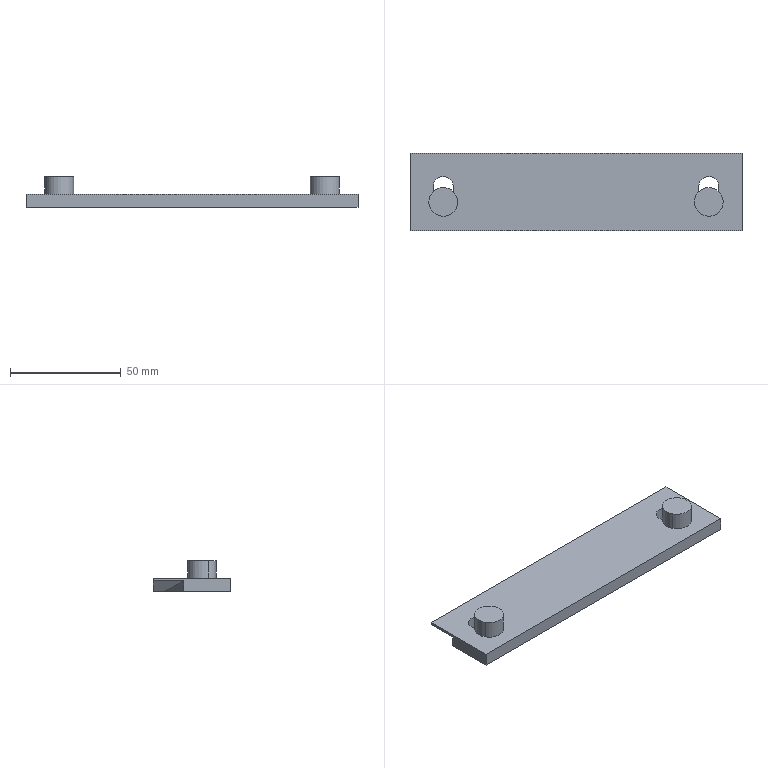Part | CATIA | 3 solids | 26 faces | box 150 x 35 x 14 mm | volume 31317 mm3 | plane 18 | cylinder 8 | commonest cylinder face diameters 9 x4 13 x4
STEP:
#1=CARTESIAN_POINT('',(-75.,-30.,38.));
#2=VERTEX_POINT('',#1);
#3=CARTESIAN_POINT('',(-75.,-30.,44.));
#4=VERTEX_POINT('',#3);
#5=CARTESIAN_POINT('',(-75.,-30.,41.));
#6=DIRECTION('',(0.,0.,1.));
#7=VECTOR('',#6,1.);
#8=LINE('',#5,#7);
#9=EDGE_CURVE('',#2,#4,#8,.T.);
#10=ORIENTED_EDGE('',*,*,#9,.F.);
#11=CARTESIAN_POINT('',(75.,-30.,38.));
#12=VERTEX_POINT('',#11);
#13=CARTESIAN_POINT('',(0.,-30.,38.));
#14=DIRECTION('',(1.,0.,0.));
#15=VECTOR('',#14,1.);
#16=LINE('',#13,#15);
#17=EDGE_CURVE('',#2,#12,#16,.T.);
#18=ORIENTED_EDGE('',*,*,#17,.T.);
#19=CARTESIAN_POINT('',(75.,-30.,44.));
#20=VERTEX_POINT('',#19);
#21=CARTESIAN_POINT('',(75.,-30.,41.));
#22=DIRECTION('',(0.,0.,1.));
#23=VECTOR('',#22,1.);
#24=LINE('',#21,#23);
#25=EDGE_CURVE('',#12,#20,#24,.T.);
#26=ORIENTED_EDGE('',*,*,#25,.T.);
#27=CARTESIAN_POINT('',(0.,-30.,44.));
#28=DIRECTION('',(1.,0.,0.));
#29=VECTOR('',#28,1.);
#30=LINE('',#27,#29);
#31=EDGE_CURVE('',#4,#20,#30,.T.);
#32=ORIENTED_EDGE('',*,*,#31,.F.);
#33=EDGE_LOOP('',(#10,#18,#26,#32));
#34=FACE_OUTER_BOUND('',#33,.T.);
#35=CARTESIAN_POINT('',(-75.,-30.,38.));
#36=DIRECTION('',(0.,-1.,0.));
#37=DIRECTION('',(1.,0.,0.));
#38=AXIS2_PLACEMENT_3D('',#35,#36,#37);
#39=PLANE('',#38);
#40=ADVANCED_FACE('',(#34),#39,.T.);
#41=CARTESIAN_POINT('',(75.,-8.66,42.874));
#42=VERTEX_POINT('',#41);
#43=CARTESIAN_POINT('',(75.,-8.66,38.));
#44=VERTEX_POINT('',#43);
#45=CARTESIAN_POINT('',(75.,-8.66,40.437));
#46=DIRECTION('',(0.,0.,-1.));
#47=VECTOR('',#46,1.);
#48=LINE('',#45,#47);
#49=EDGE_CURVE('',#42,#44,#48,.T.);
#50=ORIENTED_EDGE('',*,*,#49,.F.);
#51=CARTESIAN_POINT('',(75.,5.,42.874));
#52=VERTEX_POINT('',#51);
#53=CARTESIAN_POINT('',(75.,-1.83,42.874));
#54=DIRECTION('',(0.,1.,0.));
#55=VECTOR('',#54,1.);
#56=LINE('',#53,#55);
#57=EDGE_CURVE('',#42,#52,#56,.T.);
#58=ORIENTED_EDGE('',*,*,#57,.T.);
#59=CARTESIAN_POINT('',(75.,5.,44.));
#60=VERTEX_POINT('',#59);
#61=CARTESIAN_POINT('',(75.,5.,43.437));
#62=DIRECTION('',(0.,0.,1.));
#63=VECTOR('',#62,1.);
#64=LINE('',#61,#63);
#65=EDGE_CURVE('',#52,#60,#64,.T.);
#66=ORIENTED_EDGE('',*,*,#65,.T.);
#67=CARTESIAN_POINT('',(75.,-12.5,44.));
#68=DIRECTION('',(0.,-1.,0.));
#69=VECTOR('',#68,1.);
#70=LINE('',#67,#69);
#71=EDGE_CURVE('',#20,#60,#70,.F.);
#72=ORIENTED_EDGE('',*,*,#71,.F.);
#73=ORIENTED_EDGE('',*,*,#25,.F.);
#74=CARTESIAN_POINT('',(75.,-19.33,38.));
#75=DIRECTION('',(0.,-1.,0.));
#76=VECTOR('',#75,1.);
#77=LINE('',#74,#76);
#78=EDGE_CURVE('',#12,#44,#77,.F.);
#79=ORIENTED_EDGE('',*,*,#78,.T.);
#80=EDGE_LOOP('',(#50,#58,#66,#72,#73,#79));
#81=FACE_OUTER_BOUND('',#80,.T.);
#82=CARTESIAN_POINT('',(75.,5.,38.));
#83=DIRECTION('',(-1.,0.,0.));
#84=DIRECTION('',(0.,-1.,0.));
#85=AXIS2_PLACEMENT_3D('',#82,#83,#84);
#86=PLANE('',#85);
#87=ADVANCED_FACE('',(#81),#86,.F.);
#88=CARTESIAN_POINT('',(-75.,-8.66,42.874));
#89=VERTEX_POINT('',#88);
#90=CARTESIAN_POINT('',(-75.,5.,42.874));
#91=VERTEX_POINT('',#90);
#92=CARTESIAN_POINT('',(-75.,-1.83,42.874));
#93=DIRECTION('',(0.,1.,0.));
#94=VECTOR('',#93,1.);
#95=LINE('',#92,#94);
#96=EDGE_CURVE('',#89,#91,#95,.T.);
#97=ORIENTED_EDGE('',*,*,#96,.F.);
#98=CARTESIAN_POINT('',(-75.,-8.66,38.));
#99=VERTEX_POINT('',#98);
#100=CARTESIAN_POINT('',(-75.,-8.66,40.437));
#101=DIRECTION('',(0.,0.,-1.));
#102=VECTOR('',#101,1.);
#103=LINE('',#100,#102);
#104=EDGE_CURVE('',#89,#99,#103,.T.);
#105=ORIENTED_EDGE('',*,*,#104,.T.);
#106=CARTESIAN_POINT('',(-75.,-19.33,38.));
#107=DIRECTION('',(0.,1.,0.));
#108=VECTOR('',#107,1.);
#109=LINE('',#106,#108);
#110=EDGE_CURVE('',#99,#2,#109,.F.);
#111=ORIENTED_EDGE('',*,*,#110,.T.);
#112=ORIENTED_EDGE('',*,*,#9,.T.);
#113=CARTESIAN_POINT('',(-75.,5.,44.));
#114=VERTEX_POINT('',#113);
#115=CARTESIAN_POINT('',(-75.,-12.5,44.));
#116=DIRECTION('',(0.,1.,0.));
#117=VECTOR('',#116,1.);
#118=LINE('',#115,#117);
#119=EDGE_CURVE('',#114,#4,#118,.F.);
#120=ORIENTED_EDGE('',*,*,#119,.F.);
#121=CARTESIAN_POINT('',(-75.,5.,43.437));
#122=DIRECTION('',(0.,0.,1.));
#123=VECTOR('',#122,1.);
#124=LINE('',#121,#123);
#125=EDGE_CURVE('',#91,#114,#124,.T.);
#126=ORIENTED_EDGE('',*,*,#125,.F.);
#127=EDGE_LOOP('',(#97,#105,#111,#112,#120,#126));
#128=FACE_OUTER_BOUND('',#127,.T.);
#129=CARTESIAN_POINT('',(-75.,-30.,38.));
#130=DIRECTION('',(1.,0.,0.));
#131=DIRECTION('',(0.,1.,0.));
#132=AXIS2_PLACEMENT_3D('',#129,#130,#131);
#133=PLANE('',#132);
#134=ADVANCED_FACE('',(#128),#133,.F.);
#135=CARTESIAN_POINT('',(60.,5.,38.));
#136=VERTEX_POINT('',#135);
#137=CARTESIAN_POINT('',(-60.,5.,38.));
#138=VERTEX_POINT('',#137);
#139=CARTESIAN_POINT('',(0.,5.,38.));
#140=DIRECTION('',(-1.,0.,0.));
#141=VECTOR('',#140,1.);
#142=LINE('',#139,#141);
#143=EDGE_CURVE('',#136,#138,#142,.T.);
#144=ORIENTED_EDGE('',*,*,#143,.T.);
#145=CARTESIAN_POINT('',(-67.5,5.,40.437));
#146=DIRECTION('',(-0.9511,0.,0.309));
#147=VECTOR('',#146,1.);
#148=LINE('',#145,#147);
#149=EDGE_CURVE('',#138,#91,#148,.T.);
#150=ORIENTED_EDGE('',*,*,#149,.T.);
#151=ORIENTED_EDGE('',*,*,#125,.T.);
#152=CARTESIAN_POINT('',(0.,5.,44.));
#153=DIRECTION('',(-1.,0.,0.));
#154=VECTOR('',#153,1.);
#155=LINE('',#152,#154);
#156=EDGE_CURVE('',#60,#114,#155,.T.);
#157=ORIENTED_EDGE('',*,*,#156,.F.);
#158=ORIENTED_EDGE('',*,*,#65,.F.);
#159=CARTESIAN_POINT('',(67.5,5.,40.437));
#160=DIRECTION('',(0.9511,0.,0.309));
#161=VECTOR('',#160,1.);
#162=LINE('',#159,#161);
#163=EDGE_CURVE('',#136,#52,#162,.T.);
#164=ORIENTED_EDGE('',*,*,#163,.F.);
#165=EDGE_LOOP('',(#144,#150,#151,#157,#158,#164));
#166=FACE_OUTER_BOUND('',#165,.T.);
#167=CARTESIAN_POINT('',(75.,5.,38.));
#168=DIRECTION('',(0.,1.,0.));
#169=DIRECTION('',(-1.,0.,0.));
#170=AXIS2_PLACEMENT_3D('',#167,#168,#169);
#171=PLANE('',#170);
#172=ADVANCED_FACE('',(#166),#171,.T.);
#173=CARTESIAN_POINT('',(60.,0.,38.));
#174=VERTEX_POINT('',#173);
#175=CARTESIAN_POINT('',(75.,-8.66,42.874));
#176=CARTESIAN_POINT('',(60.,0.,38.));
#177=B_SPLINE_CURVE_WITH_KNOTS('',1,(#175,#176),.UNSPECIFIED.,.F.,.U.,(2,2),(-2.999,14.994),.UNSPECIFIED.);
#178=EDGE_CURVE('',#174,#42,#177,.F.);
#179=ORIENTED_EDGE('',*,*,#178,.T.);
#180=ORIENTED_EDGE('',*,*,#49,.T.);
#181=CARTESIAN_POINT('',(72.5,-7.217,38.));
#182=DIRECTION('',(0.866,-0.5,0.));
#183=VECTOR('',#182,1.);
#184=LINE('',#181,#183);
#185=EDGE_CURVE('',#174,#44,#184,.T.);
#186=ORIENTED_EDGE('',*,*,#185,.F.);
#187=EDGE_LOOP('',(#179,#180,#186));
#188=FACE_OUTER_BOUND('',#187,.T.);
#189=CARTESIAN_POINT('',(60.,0.,38.));
#190=DIRECTION('',(0.5,0.866,0.));
#191=DIRECTION('',(0.,0.,1.));
#192=AXIS2_PLACEMENT_3D('',#189,#190,#191);
#193=PLANE('',#192);
#194=ADVANCED_FACE('',(#188),#193,.T.);
#195=ORIENTED_EDGE('',*,*,#163,.T.);
#196=ORIENTED_EDGE('',*,*,#57,.F.);
#197=ORIENTED_EDGE('',*,*,#178,.F.);
#198=CARTESIAN_POINT('',(60.,5.,38.));
#199=DIRECTION('',(0.,-1.,0.));
#200=VECTOR('',#199,1.);
#201=LINE('',#198,#200);
#202=EDGE_CURVE('',#174,#136,#201,.F.);
#203=ORIENTED_EDGE('',*,*,#202,.T.);
#204=EDGE_LOOP('',(#195,#196,#197,#203));
#205=FACE_OUTER_BOUND('',#204,.T.);
#206=CARTESIAN_POINT('',(60.,10.,38.));
#207=DIRECTION('',(-0.309,0.,0.9511));
#208=DIRECTION('',(0.,-1.,0.));
#209=AXIS2_PLACEMENT_3D('',#206,#207,#208);
#210=PLANE('',#209);
#211=ADVANCED_FACE('',(#205),#210,.F.);
#212=CARTESIAN_POINT('',(-60.,0.,38.));
#213=VERTEX_POINT('',#212);
#214=CARTESIAN_POINT('',(-72.5,-7.217,38.));
#215=DIRECTION('',(-0.866,-0.5,0.));
#216=VECTOR('',#215,1.);
#217=LINE('',#214,#216);
#218=EDGE_CURVE('',#213,#99,#217,.T.);
#219=ORIENTED_EDGE('',*,*,#218,.T.);
#220=ORIENTED_EDGE('',*,*,#104,.F.);
#221=CARTESIAN_POINT('',(-75.,-8.66,42.874));
#222=CARTESIAN_POINT('',(-60.,0.,38.));
#223=B_SPLINE_CURVE_WITH_KNOTS('',1,(#221,#222),.UNSPECIFIED.,.F.,.U.,(2,2),(-2.999,14.994),.UNSPECIFIED.);
#224=EDGE_CURVE('',#213,#89,#223,.F.);
#225=ORIENTED_EDGE('',*,*,#224,.F.);
#226=EDGE_LOOP('',(#219,#220,#225));
#227=FACE_OUTER_BOUND('',#226,.T.);
#228=CARTESIAN_POINT('',(-60.,0.,38.));
#229=DIRECTION('',(0.5,-0.866,0.));
#230=DIRECTION('',(0.,0.,1.));
#231=AXIS2_PLACEMENT_3D('',#228,#229,#230);
#232=PLANE('',#231);
#233=ADVANCED_FACE('',(#227),#232,.F.);
#234=CARTESIAN_POINT('',(-60.,5.,38.));
#235=DIRECTION('',(0.,-1.,0.));
#236=VECTOR('',#235,1.);
#237=LINE('',#234,#236);
#238=EDGE_CURVE('',#213,#138,#237,.F.);
#239=ORIENTED_EDGE('',*,*,#238,.F.);
#240=ORIENTED_EDGE('',*,*,#224,.T.);
#241=ORIENTED_EDGE('',*,*,#96,.T.);
#242=ORIENTED_EDGE('',*,*,#149,.F.);
#243=EDGE_LOOP('',(#239,#240,#241,#242));
#244=FACE_OUTER_BOUND('',#243,.T.);
#245=CARTESIAN_POINT('',(-60.,10.,38.));
#246=DIRECTION('',(-0.309,0.,-0.9511));
#247=DIRECTION('',(0.,-1.,0.));
#248=AXIS2_PLACEMENT_3D('',#245,#246,#247);
#249=PLANE('',#248);
#250=ADVANCED_FACE('',(#244),#249,.T.);
#251=ORIENTED_EDGE('',*,*,#143,.F.);
#252=ORIENTED_EDGE('',*,*,#202,.F.);
#253=ORIENTED_EDGE('',*,*,#185,.T.);
#254=ORIENTED_EDGE('',*,*,#78,.F.);
#255=ORIENTED_EDGE('',*,*,#17,.F.);
#256=ORIENTED_EDGE('',*,*,#110,.F.);
#257=ORIENTED_EDGE('',*,*,#218,.F.);
#258=ORIENTED_EDGE('',*,*,#238,.T.);
#259=EDGE_LOOP('',(#251,#252,#253,#254,#255,#256,#257,#258));
#260=FACE_OUTER_BOUND('',#259,.T.);
#261=CARTESIAN_POINT('',(-55.5,-10.,38.));
#262=VERTEX_POINT('',#261);
#263=CARTESIAN_POINT('',(-55.5,-17.,38.));
#264=VERTEX_POINT('',#263);
#265=CARTESIAN_POINT('',(-55.5,-13.5,38.));
#266=DIRECTION('',(0.,-1.,0.));
#267=VECTOR('',#266,1.);
#268=LINE('',#265,#267);
#269=EDGE_CURVE('',#262,#264,#268,.T.);
#270=ORIENTED_EDGE('',*,*,#269,.F.);
#271=CARTESIAN_POINT('',(-64.5,-10.,38.));
#272=VERTEX_POINT('',#271);
#273=CARTESIAN_POINT('',(-60.,-10.,38.));
#274=DIRECTION('',(0.,0.,1.));
#275=AXIS2_PLACEMENT_3D('',#273,#274,$);
#276=CIRCLE('',#275,4.5);
#277=EDGE_CURVE('',#262,#272,#276,.T.);
#278=ORIENTED_EDGE('',*,*,#277,.T.);
#279=CARTESIAN_POINT('',(-64.5,-17.,38.));
#280=VERTEX_POINT('',#279);
#281=CARTESIAN_POINT('',(-64.5,-13.5,38.));
#282=DIRECTION('',(0.,-1.,0.));
#283=VECTOR('',#282,1.);
#284=LINE('',#281,#283);
#285=EDGE_CURVE('',#272,#280,#284,.T.);
#286=ORIENTED_EDGE('',*,*,#285,.T.);
#287=CARTESIAN_POINT('',(-60.,-17.,38.));
#288=DIRECTION('',(0.,0.,1.));
#289=AXIS2_PLACEMENT_3D('',#287,#288,$);
#290=CIRCLE('',#289,4.5);
#291=EDGE_CURVE('',#280,#264,#290,.T.);
#292=ORIENTED_EDGE('',*,*,#291,.T.);
#293=EDGE_LOOP('',(#270,#278,#286,#292));
#294=FACE_BOUND('',#293,.T.);
#295=CARTESIAN_POINT('',(64.5,-10.,38.));
#296=VERTEX_POINT('',#295);
#297=CARTESIAN_POINT('',(55.5,-10.,38.));
#298=VERTEX_POINT('',#297);
#299=CARTESIAN_POINT('',(60.,-10.,38.));
#300=DIRECTION('',(0.,0.,1.));
#301=AXIS2_PLACEMENT_3D('',#299,#300,$);
#302=CIRCLE('',#301,4.5);
#303=EDGE_CURVE('',#296,#298,#302,.T.);
#304=ORIENTED_EDGE('',*,*,#303,.T.);
#305=CARTESIAN_POINT('',(55.5,-17.,38.));
#306=VERTEX_POINT('',#305);
#307=CARTESIAN_POINT('',(55.5,-13.5,38.));
#308=DIRECTION('',(0.,-1.,0.));
#309=VECTOR('',#308,1.);
#310=LINE('',#307,#309);
#311=EDGE_CURVE('',#298,#306,#310,.T.);
#312=ORIENTED_EDGE('',*,*,#311,.T.);
#313=CARTESIAN_POINT('',(64.5,-17.,38.));
#314=VERTEX_POINT('',#313);
#315=CARTESIAN_POINT('',(60.,-17.,38.));
#316=DIRECTION('',(0.,0.,1.));
#317=AXIS2_PLACEMENT_3D('',#315,#316,$);
#318=CIRCLE('',#317,4.5);
#319=EDGE_CURVE('',#306,#314,#318,.T.);
#320=ORIENTED_EDGE('',*,*,#319,.T.);
#321=CARTESIAN_POINT('',(64.5,-13.5,38.));
#322=DIRECTION('',(0.,-1.,0.));
#323=VECTOR('',#322,1.);
#324=LINE('',#321,#323);
#325=EDGE_CURVE('',#296,#314,#324,.T.);
#326=ORIENTED_EDGE('',*,*,#325,.F.);
#327=EDGE_LOOP('',(#304,#312,#320,#326));
#328=FACE_BOUND('',#327,.T.);
#329=CARTESIAN_POINT('',(0.,0.,38.));
#330=DIRECTION('',(0.,0.,1.));
#331=DIRECTION('',(1.,0.,0.));
#332=AXIS2_PLACEMENT_3D('',#329,#330,#331);
#333=PLANE('',#332);
#334=ADVANCED_FACE('',(#260,#294,#328),#333,.F.);
#335=ORIENTED_EDGE('',*,*,#156,.T.);
#336=ORIENTED_EDGE('',*,*,#119,.T.);
#337=ORIENTED_EDGE('',*,*,#31,.T.);
#338=ORIENTED_EDGE('',*,*,#71,.T.);
#339=EDGE_LOOP('',(#335,#336,#337,#338));
#340=FACE_OUTER_BOUND('',#339,.T.);
#341=CARTESIAN_POINT('',(-55.5,-17.,44.));
#342=VERTEX_POINT('',#341);
#343=CARTESIAN_POINT('',(-55.5,-10.,44.));
#344=VERTEX_POINT('',#343);
#345=CARTESIAN_POINT('',(-55.5,-13.5,44.));
#346=DIRECTION('',(0.,-1.,0.));
#347=VECTOR('',#346,1.);
#348=LINE('',#345,#347);
#349=EDGE_CURVE('',#342,#344,#348,.F.);
#350=ORIENTED_EDGE('',*,*,#349,.F.);
#351=CARTESIAN_POINT('',(-64.5,-17.,44.));
#352=VERTEX_POINT('',#351);
#353=CARTESIAN_POINT('',(-60.,-17.,44.));
#354=DIRECTION('',(0.,0.,1.));
#355=AXIS2_PLACEMENT_3D('',#353,#354,$);
#356=CIRCLE('',#355,4.5);
#357=EDGE_CURVE('',#352,#342,#356,.T.);
#358=ORIENTED_EDGE('',*,*,#357,.F.);
#359=CARTESIAN_POINT('',(-64.5,-10.,44.));
#360=VERTEX_POINT('',#359);
#361=CARTESIAN_POINT('',(-64.5,-13.5,44.));
#362=DIRECTION('',(0.,-1.,0.));
#363=VECTOR('',#362,1.);
#364=LINE('',#361,#363);
#365=EDGE_CURVE('',#360,#352,#364,.T.);
#366=ORIENTED_EDGE('',*,*,#365,.F.);
#367=CARTESIAN_POINT('',(-60.,-10.,44.));
#368=DIRECTION('',(0.,0.,1.));
#369=AXIS2_PLACEMENT_3D('',#367,#368,$);
#370=CIRCLE('',#369,4.5);
#371=EDGE_CURVE('',#344,#360,#370,.T.);
#372=ORIENTED_EDGE('',*,*,#371,.F.);
#373=EDGE_LOOP('',(#350,#358,#366,#372));
#374=FACE_BOUND('',#373,.T.);
#375=CARTESIAN_POINT('',(64.5,-10.,44.));
#376=VERTEX_POINT('',#375);
#377=CARTESIAN_POINT('',(55.5,-10.,44.));
#378=VERTEX_POINT('',#377);
#379=CARTESIAN_POINT('',(60.,-10.,44.));
#380=DIRECTION('',(0.,0.,1.));
#381=AXIS2_PLACEMENT_3D('',#379,#380,$);
#382=CIRCLE('',#381,4.5);
#383=EDGE_CURVE('',#376,#378,#382,.T.);
#384=ORIENTED_EDGE('',*,*,#383,.F.);
#385=CARTESIAN_POINT('',(64.5,-17.,44.));
#386=VERTEX_POINT('',#385);
#387=CARTESIAN_POINT('',(64.5,-13.5,44.));
#388=DIRECTION('',(0.,-1.,0.));
#389=VECTOR('',#388,1.);
#390=LINE('',#387,#389);
#391=EDGE_CURVE('',#386,#376,#390,.F.);
#392=ORIENTED_EDGE('',*,*,#391,.F.);
#393=CARTESIAN_POINT('',(55.5,-17.,44.));
#394=VERTEX_POINT('',#393);
#395=CARTESIAN_POINT('',(60.,-17.,44.));
#396=DIRECTION('',(0.,0.,1.));
#397=AXIS2_PLACEMENT_3D('',#395,#396,$);
#398=CIRCLE('',#397,4.5);
#399=EDGE_CURVE('',#394,#386,#398,.T.);
#400=ORIENTED_EDGE('',*,*,#399,.F.);
#401=CARTESIAN_POINT('',(55.5,-13.5,44.));
#402=DIRECTION('',(0.,-1.,0.));
#403=VECTOR('',#402,1.);
#404=LINE('',#401,#403);
#405=EDGE_CURVE('',#378,#394,#404,.T.);
#406=ORIENTED_EDGE('',*,*,#405,.F.);
#407=EDGE_LOOP('',(#384,#392,#400,#406));
#408=FACE_BOUND('',#407,.T.);
#409=CARTESIAN_POINT('',(0.,0.,44.));
#410=DIRECTION('',(0.,0.,1.));
#411=DIRECTION('',(1.,0.,0.));
#412=AXIS2_PLACEMENT_3D('',#409,#410,#411);
#413=PLANE('',#412);
#414=ADVANCED_FACE('',(#340,#374,#408),#413,.T.);
#415=ORIENTED_EDGE('',*,*,#303,.F.);
#416=CARTESIAN_POINT('',(64.5,-10.,34.));
#417=DIRECTION('',(0.,0.,1.));
#418=VECTOR('',#417,1.);
#419=LINE('',#416,#418);
#420=EDGE_CURVE('',#376,#296,#419,.F.);
#421=ORIENTED_EDGE('',*,*,#420,.F.);
#422=ORIENTED_EDGE('',*,*,#383,.T.);
#423=CARTESIAN_POINT('',(55.5,-10.,34.));
#424=DIRECTION('',(0.,0.,1.));
#425=VECTOR('',#424,1.);
#426=LINE('',#423,#425);
#427=EDGE_CURVE('',#378,#298,#426,.F.);
#428=ORIENTED_EDGE('',*,*,#427,.T.);
#429=EDGE_LOOP('',(#415,#421,#422,#428));
#430=FACE_OUTER_BOUND('',#429,.T.);
#431=CARTESIAN_POINT('',(60.,-10.,34.));
#432=DIRECTION('',(0.,0.,1.));
#433=DIRECTION('',(1.,0.,0.));
#434=AXIS2_PLACEMENT_3D('',#431,#432,#433);
#435=CYLINDRICAL_SURFACE('',#434,4.5);
#436=ADVANCED_FACE('',(#430),#435,.F.);
#437=ORIENTED_EDGE('',*,*,#427,.F.);
#438=ORIENTED_EDGE('',*,*,#405,.T.);
#439=CARTESIAN_POINT('',(55.5,-17.,41.));
#440=DIRECTION('',(0.,0.,-1.));
#441=VECTOR('',#440,1.);
#442=LINE('',#439,#441);
#443=EDGE_CURVE('',#394,#306,#442,.T.);
#444=ORIENTED_EDGE('',*,*,#443,.T.);
#445=ORIENTED_EDGE('',*,*,#311,.F.);
#446=EDGE_LOOP('',(#437,#438,#444,#445));
#447=FACE_OUTER_BOUND('',#446,.T.);
#448=CARTESIAN_POINT('',(55.5,-10.,44.));
#449=DIRECTION('',(1.,0.,0.));
#450=DIRECTION('',(0.,-1.,0.));
#451=AXIS2_PLACEMENT_3D('',#448,#449,#450);
#452=PLANE('',#451);
#453=ADVANCED_FACE('',(#447),#452,.T.);
#454=ORIENTED_EDGE('',*,*,#325,.T.);
#455=CARTESIAN_POINT('',(64.5,-17.,41.));
#456=DIRECTION('',(0.,0.,-1.));
#457=VECTOR('',#456,1.);
#458=LINE('',#455,#457);
#459=EDGE_CURVE('',#386,#314,#458,.T.);
#460=ORIENTED_EDGE('',*,*,#459,.F.);
#461=ORIENTED_EDGE('',*,*,#391,.T.);
#462=ORIENTED_EDGE('',*,*,#420,.T.);
#463=EDGE_LOOP('',(#454,#460,#461,#462));
#464=FACE_OUTER_BOUND('',#463,.T.);
#465=CARTESIAN_POINT('',(64.5,-10.,44.));
#466=DIRECTION('',(1.,0.,0.));
#467=DIRECTION('',(0.,-1.,0.));
#468=AXIS2_PLACEMENT_3D('',#465,#466,#467);
#469=PLANE('',#468);
#470=ADVANCED_FACE('',(#464),#469,.F.);
#471=ORIENTED_EDGE('',*,*,#319,.F.);
#472=ORIENTED_EDGE('',*,*,#443,.F.);
#473=ORIENTED_EDGE('',*,*,#399,.T.);
#474=ORIENTED_EDGE('',*,*,#459,.T.);
#475=EDGE_LOOP('',(#471,#472,#473,#474));
#476=FACE_OUTER_BOUND('',#475,.T.);
#477=CARTESIAN_POINT('',(60.,-17.,34.));
#478=DIRECTION('',(0.,0.,1.));
#479=DIRECTION('',(-1.,0.,0.));
#480=AXIS2_PLACEMENT_3D('',#477,#478,#479);
#481=CYLINDRICAL_SURFACE('',#480,4.5);
#482=ADVANCED_FACE('',(#476),#481,.F.);
#483=ORIENTED_EDGE('',*,*,#269,.T.);
#484=CARTESIAN_POINT('',(-55.5,-17.,41.));
#485=DIRECTION('',(0.,0.,-1.));
#486=VECTOR('',#485,1.);
#487=LINE('',#484,#486);
#488=EDGE_CURVE('',#342,#264,#487,.T.);
#489=ORIENTED_EDGE('',*,*,#488,.F.);
#490=ORIENTED_EDGE('',*,*,#349,.T.);
#491=CARTESIAN_POINT('',(-55.5,-10.,41.));
#492=DIRECTION('',(0.,0.,-1.));
#493=VECTOR('',#492,1.);
#494=LINE('',#491,#493);
#495=EDGE_CURVE('',#344,#262,#494,.T.);
#496=ORIENTED_EDGE('',*,*,#495,.T.);
#497=EDGE_LOOP('',(#483,#489,#490,#496));
#498=FACE_OUTER_BOUND('',#497,.T.);
#499=CARTESIAN_POINT('',(-55.5,-10.,44.));
#500=DIRECTION('',(1.,0.,0.));
#501=DIRECTION('',(0.,-1.,0.));
#502=AXIS2_PLACEMENT_3D('',#499,#500,#501);
#503=PLANE('',#502);
#504=ADVANCED_FACE('',(#498),#503,.F.);
#505=ORIENTED_EDGE('',*,*,#277,.F.);
#506=ORIENTED_EDGE('',*,*,#495,.F.);
#507=ORIENTED_EDGE('',*,*,#371,.T.);
#508=CARTESIAN_POINT('',(-64.5,-10.,34.));
#509=DIRECTION('',(0.,0.,1.));
#510=VECTOR('',#509,1.);
#511=LINE('',#508,#510);
#512=EDGE_CURVE('',#360,#272,#511,.F.);
#513=ORIENTED_EDGE('',*,*,#512,.T.);
#514=EDGE_LOOP('',(#505,#506,#507,#513));
#515=FACE_OUTER_BOUND('',#514,.T.);
#516=CARTESIAN_POINT('',(-60.,-10.,34.));
#517=DIRECTION('',(0.,0.,1.));
#518=DIRECTION('',(1.,0.,0.));
#519=AXIS2_PLACEMENT_3D('',#516,#517,#518);
#520=CYLINDRICAL_SURFACE('',#519,4.5);
#521=ADVANCED_FACE('',(#515),#520,.F.);
#522=ORIENTED_EDGE('',*,*,#291,.F.);
#523=CARTESIAN_POINT('',(-64.5,-17.,34.));
#524=DIRECTION('',(0.,0.,1.));
#525=VECTOR('',#524,1.);
#526=LINE('',#523,#525);
#527=EDGE_CURVE('',#352,#280,#526,.F.);
#528=ORIENTED_EDGE('',*,*,#527,.F.);
#529=ORIENTED_EDGE('',*,*,#357,.T.);
#530=ORIENTED_EDGE('',*,*,#488,.T.);
#531=EDGE_LOOP('',(#522,#528,#529,#530));
#532=FACE_OUTER_BOUND('',#531,.T.);
#533=CARTESIAN_POINT('',(-60.,-17.,34.));
#534=DIRECTION('',(0.,0.,1.));
#535=DIRECTION('',(-1.,0.,0.));
#536=AXIS2_PLACEMENT_3D('',#533,#534,#535);
#537=CYLINDRICAL_SURFACE('',#536,4.5);
#538=ADVANCED_FACE('',(#532),#537,.F.);
#539=ORIENTED_EDGE('',*,*,#512,.F.);
#540=ORIENTED_EDGE('',*,*,#365,.T.);
#541=ORIENTED_EDGE('',*,*,#527,.T.);
#542=ORIENTED_EDGE('',*,*,#285,.F.);
#543=EDGE_LOOP('',(#539,#540,#541,#542));
#544=FACE_OUTER_BOUND('',#543,.T.);
#545=CARTESIAN_POINT('',(-64.5,-10.,44.));
#546=DIRECTION('',(1.,0.,0.));
#547=DIRECTION('',(0.,-1.,0.));
#548=AXIS2_PLACEMENT_3D('',#545,#546,#547);
#549=PLANE('',#548);
#550=ADVANCED_FACE('',(#544),#549,.T.);
#551=CLOSED_SHELL('',(#40,#87,#134,#172,#194,#211,#233,#250,#334,#414,#436,#453,#470,#482,#504,#521,#538,#550));
#552=MANIFOLD_SOLID_BREP('',#551);
#553=CARTESIAN_POINT('',(-54.296,-13.884,52.));
#554=VERTEX_POINT('',#553);
#555=CARTESIAN_POINT('',(-65.704,-20.116,52.));
#556=VERTEX_POINT('',#555);
#557=CARTESIAN_POINT('',(-60.,-17.,52.));
#558=DIRECTION('',(0.,0.,1.));
#559=AXIS2_PLACEMENT_3D('',#557,#558,$);
#560=CIRCLE('',#559,6.5);
#561=EDGE_CURVE('',#554,#556,#560,.T.);
#562=ORIENTED_EDGE('',*,*,#561,.T.);
#563=CARTESIAN_POINT('',(-60.,-17.,52.));
#564=DIRECTION('',(0.,0.,1.));
#565=AXIS2_PLACEMENT_3D('',#563,#564,$);
#566=CIRCLE('',#565,6.5);
#567=EDGE_CURVE('',#556,#554,#566,.T.);
#568=ORIENTED_EDGE('',*,*,#567,.T.);
#569=EDGE_LOOP('',(#562,#568));
#570=FACE_OUTER_BOUND('',#569,.T.);
#571=CARTESIAN_POINT('',(-60.,-17.,52.));
#572=DIRECTION('',(0.,0.,1.));
#573=DIRECTION('',(1.,0.,0.));
#574=AXIS2_PLACEMENT_3D('',#571,#572,#573);
#575=PLANE('',#574);
#576=ADVANCED_FACE('',(#570),#575,.T.);
#577=CARTESIAN_POINT('',(-65.704,-20.116,44.));
#578=VERTEX_POINT('',#577);
#579=CARTESIAN_POINT('',(-65.704,-20.116,47.8));
#580=DIRECTION('',(0.,0.,1.));
#581=VECTOR('',#580,1.);
#582=LINE('',#579,#581);
#583=EDGE_CURVE('',#556,#578,#582,.F.);
#584=ORIENTED_EDGE('',*,*,#583,.F.);
#585=ORIENTED_EDGE('',*,*,#561,.F.);
#586=CARTESIAN_POINT('',(-54.296,-13.884,44.));
#587=VERTEX_POINT('',#586);
#588=CARTESIAN_POINT('',(-54.296,-13.884,47.8));
#589=DIRECTION('',(0.,0.,1.));
#590=VECTOR('',#589,1.);
#591=LINE('',#588,#590);
#592=EDGE_CURVE('',#554,#587,#591,.F.);
#593=ORIENTED_EDGE('',*,*,#592,.T.);
#594=CARTESIAN_POINT('',(-60.,-17.,44.));
#595=DIRECTION('',(0.,0.,1.));
#596=AXIS2_PLACEMENT_3D('',#594,#595,$);
#597=CIRCLE('',#596,6.5);
#598=EDGE_CURVE('',#587,#578,#597,.T.);
#599=ORIENTED_EDGE('',*,*,#598,.T.);
#600=EDGE_LOOP('',(#584,#585,#593,#599));
#601=FACE_OUTER_BOUND('',#600,.T.);
#602=CARTESIAN_POINT('',(-60.,-17.,44.1));
#603=DIRECTION('',(0.,0.,1.));
#604=DIRECTION('',(0.8776,0.4794,0.));
#605=AXIS2_PLACEMENT_3D('',#602,#603,#604);
#606=CYLINDRICAL_SURFACE('',#605,6.5);
#607=ADVANCED_FACE('',(#601),#606,.T.);
#608=ORIENTED_EDGE('',*,*,#592,.F.);
#609=ORIENTED_EDGE('',*,*,#567,.F.);
#610=ORIENTED_EDGE('',*,*,#583,.T.);
#611=CARTESIAN_POINT('',(-60.,-17.,44.));
#612=DIRECTION('',(0.,0.,1.));
#613=AXIS2_PLACEMENT_3D('',#611,#612,$);
#614=CIRCLE('',#613,6.5);
#615=EDGE_CURVE('',#578,#587,#614,.T.);
#616=ORIENTED_EDGE('',*,*,#615,.T.);
#617=EDGE_LOOP('',(#608,#609,#610,#616));
#618=FACE_OUTER_BOUND('',#617,.T.);
#619=ADVANCED_FACE('',(#618),#606,.T.);
#620=ORIENTED_EDGE('',*,*,#598,.F.);
#621=ORIENTED_EDGE('',*,*,#615,.F.);
#622=EDGE_LOOP('',(#620,#621));
#623=FACE_OUTER_BOUND('',#622,.T.);
#624=ADVANCED_FACE('',(#623),#413,.F.);
#625=CLOSED_SHELL('',(#576,#607,#619,#624));
#626=MANIFOLD_SOLID_BREP('',#625);
#627=CARTESIAN_POINT('',(65.704,-13.884,52.));
#628=VERTEX_POINT('',#627);
#629=CARTESIAN_POINT('',(54.296,-20.116,52.));
#630=VERTEX_POINT('',#629);
#631=CARTESIAN_POINT('',(60.,-17.,52.));
#632=DIRECTION('',(0.,0.,1.));
#633=AXIS2_PLACEMENT_3D('',#631,#632,$);
#634=CIRCLE('',#633,6.5);
#635=EDGE_CURVE('',#628,#630,#634,.T.);
#636=ORIENTED_EDGE('',*,*,#635,.T.);
#637=CARTESIAN_POINT('',(60.,-17.,52.));
#638=DIRECTION('',(0.,0.,1.));
#639=AXIS2_PLACEMENT_3D('',#637,#638,$);
#640=CIRCLE('',#639,6.5);
#641=EDGE_CURVE('',#630,#628,#640,.T.);
#642=ORIENTED_EDGE('',*,*,#641,.T.);
#643=EDGE_LOOP('',(#636,#642));
#644=FACE_OUTER_BOUND('',#643,.T.);
#645=ADVANCED_FACE('',(#644),#575,.T.);
#646=CARTESIAN_POINT('',(54.296,-20.116,44.));
#647=VERTEX_POINT('',#646);
#648=CARTESIAN_POINT('',(54.296,-20.116,47.8));
#649=DIRECTION('',(0.,0.,1.));
#650=VECTOR('',#649,1.);
#651=LINE('',#648,#650);
#652=EDGE_CURVE('',#630,#647,#651,.F.);
#653=ORIENTED_EDGE('',*,*,#652,.F.);
#654=ORIENTED_EDGE('',*,*,#635,.F.);
#655=CARTESIAN_POINT('',(65.704,-13.884,44.));
#656=VERTEX_POINT('',#655);
#657=CARTESIAN_POINT('',(65.704,-13.884,47.8));
#658=DIRECTION('',(0.,0.,1.));
#659=VECTOR('',#658,1.);
#660=LINE('',#657,#659);
#661=EDGE_CURVE('',#628,#656,#660,.F.);
#662=ORIENTED_EDGE('',*,*,#661,.T.);
#663=CARTESIAN_POINT('',(60.,-17.,44.));
#664=DIRECTION('',(0.,0.,1.));
#665=AXIS2_PLACEMENT_3D('',#663,#664,$);
#666=CIRCLE('',#665,6.5);
#667=EDGE_CURVE('',#656,#647,#666,.T.);
#668=ORIENTED_EDGE('',*,*,#667,.T.);
#669=EDGE_LOOP('',(#653,#654,#662,#668));
#670=FACE_OUTER_BOUND('',#669,.T.);
#671=CARTESIAN_POINT('',(60.,-17.,44.1));
#672=DIRECTION('',(0.,0.,1.));
#673=DIRECTION('',(0.8776,0.4794,0.));
#674=AXIS2_PLACEMENT_3D('',#671,#672,#673);
#675=CYLINDRICAL_SURFACE('',#674,6.5);
#676=ADVANCED_FACE('',(#670),#675,.T.);
#677=ORIENTED_EDGE('',*,*,#661,.F.);
#678=ORIENTED_EDGE('',*,*,#641,.F.);
#679=ORIENTED_EDGE('',*,*,#652,.T.);
#680=CARTESIAN_POINT('',(60.,-17.,44.));
#681=DIRECTION('',(0.,0.,1.));
#682=AXIS2_PLACEMENT_3D('',#680,#681,$);
#683=CIRCLE('',#682,6.5);
#684=EDGE_CURVE('',#647,#656,#683,.T.);
#685=ORIENTED_EDGE('',*,*,#684,.T.);
#686=EDGE_LOOP('',(#677,#678,#679,#685));
#687=FACE_OUTER_BOUND('',#686,.T.);
#688=ADVANCED_FACE('',(#687),#675,.T.);
#689=ORIENTED_EDGE('',*,*,#667,.F.);
#690=ORIENTED_EDGE('',*,*,#684,.F.);
#691=EDGE_LOOP('',(#689,#690));
#692=FACE_OUTER_BOUND('',#691,.T.);
#693=ADVANCED_FACE('',(#692),#413,.F.);
#694=CLOSED_SHELL('',(#645,#676,#688,#693));
#695=MANIFOLD_SOLID_BREP('',#694);
#696=(LENGTH_UNIT()NAMED_UNIT(*)SI_UNIT(.MILLI.,.METRE.));
#697=UNCERTAINTY_MEASURE_WITH_UNIT(LENGTH_MEASURE(0.005),#696,'','');
#698=(NAMED_UNIT(*)PLANE_ANGLE_UNIT()SI_UNIT($,.RADIAN.));
#699=(NAMED_UNIT(*)SI_UNIT($,.STERADIAN.)SOLID_ANGLE_UNIT());
#700=(GEOMETRIC_REPRESENTATION_CONTEXT(3)GLOBAL_UNCERTAINTY_ASSIGNED_CONTEXT((#697))GLOBAL_UNIT_ASSIGNED_CONTEXT((#696,#698,#699))REPRESENTATION_CONTEXT('',''));
#701=ADVANCED_BREP_SHAPE_REPRESENTATION('',(#552,#626,#695),#700);